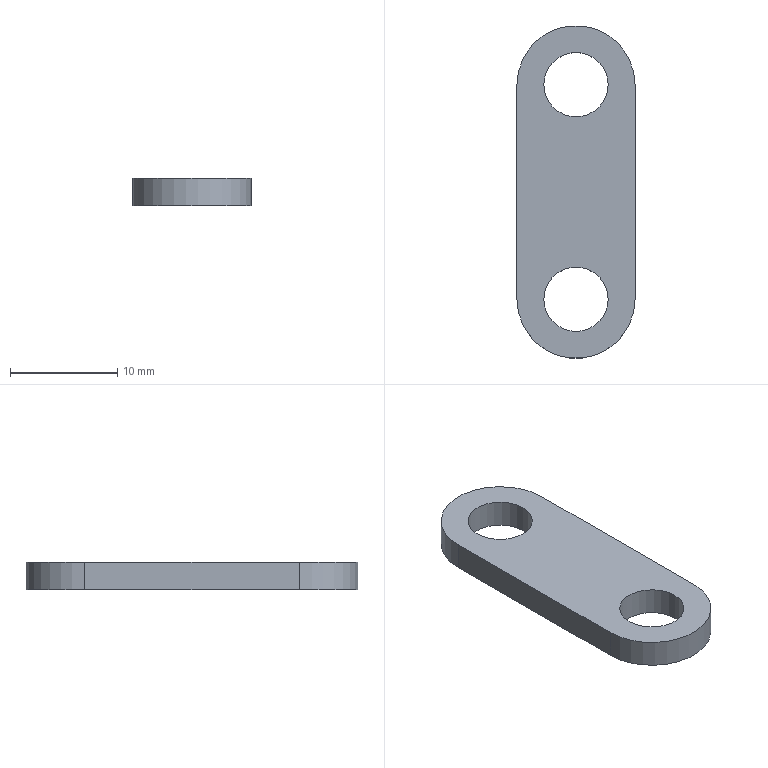Part | NX | features DATUM_CSYS 2, EXTRUDE 1, SKETCH 1 | 1 solid | 8 faces | box 11 x 31 x 2.6 mm | volume 672.06 mm3 | plane 4 | cylinder 4 | commonest cylinder face diameters 6 x2 11 x2
STEP:
#1=CARTESIAN_POINT('',(-5.5,10.,0.));
#2=VERTEX_POINT('',#1);
#3=CARTESIAN_POINT('',(-5.5,-10.,0.));
#4=VERTEX_POINT('',#3);
#5=CARTESIAN_POINT('',(-5.5,10.,0.));
#6=DIRECTION('',(0.,-1.,0.));
#7=VECTOR('',#6,1000.);
#8=LINE('',#5,#7);
#9=EDGE_CURVE('',#2,#4,#8,.T.);
#10=ORIENTED_EDGE('',*,*,#9,.T.);
#11=CARTESIAN_POINT('',(-5.5,-10.,2.6));
#12=VERTEX_POINT('',#11);
#13=CARTESIAN_POINT('',(-5.5,-10.,2.6));
#14=DIRECTION('',(0.,0.,-1.));
#15=VECTOR('',#14,1000.);
#16=LINE('',#13,#15);
#17=EDGE_CURVE('',#12,#4,#16,.T.);
#18=ORIENTED_EDGE('',*,*,#17,.F.);
#19=CARTESIAN_POINT('',(-5.5,10.,2.6));
#20=VERTEX_POINT('',#19);
#21=CARTESIAN_POINT('',(-5.5,10.,2.6));
#22=DIRECTION('',(0.,-1.,0.));
#23=VECTOR('',#22,1000.);
#24=LINE('',#21,#23);
#25=EDGE_CURVE('',#20,#12,#24,.T.);
#26=ORIENTED_EDGE('',*,*,#25,.F.);
#27=CARTESIAN_POINT('',(-5.5,10.,2.6));
#28=DIRECTION('',(0.,0.,-1.));
#29=VECTOR('',#28,1000.);
#30=LINE('',#27,#29);
#31=EDGE_CURVE('',#20,#2,#30,.T.);
#32=ORIENTED_EDGE('',*,*,#31,.T.);
#33=EDGE_LOOP('',(#10,#18,#26,#32));
#34=FACE_BOUND('',#33,.T.);
#35=CARTESIAN_POINT('',(-5.5,10.,2.6));
#36=DIRECTION('',(1.,0.,0.));
#37=DIRECTION('',(0.,0.,-1.));
#38=AXIS2_PLACEMENT_3D('',#35,#36,#37);
#39=PLANE('',#38);
#40=ADVANCED_FACE('',(#34),#39,.F.);
#41=CARTESIAN_POINT('',(5.5,-10.,0.));
#42=VERTEX_POINT('',#41);
#43=CARTESIAN_POINT('',(0.,-10.,0.));
#44=DIRECTION('',(0.,0.,1.));
#45=DIRECTION('',(1.,0.,0.));
#46=AXIS2_PLACEMENT_3D('',#43,#44,#45);
#47=CIRCLE('',#46,5.5);
#48=EDGE_CURVE('',#4,#42,#47,.T.);
#49=ORIENTED_EDGE('',*,*,#48,.T.);
#50=CARTESIAN_POINT('',(5.5,-10.,2.6));
#51=VERTEX_POINT('',#50);
#52=CARTESIAN_POINT('',(5.5,-10.,2.6));
#53=DIRECTION('',(0.,0.,-1.));
#54=VECTOR('',#53,1000.);
#55=LINE('',#52,#54);
#56=EDGE_CURVE('',#51,#42,#55,.T.);
#57=ORIENTED_EDGE('',*,*,#56,.F.);
#58=CARTESIAN_POINT('',(0.,-10.,2.6));
#59=DIRECTION('',(0.,0.,1.));
#60=DIRECTION('',(1.,0.,0.));
#61=AXIS2_PLACEMENT_3D('',#58,#59,#60);
#62=CIRCLE('',#61,5.5);
#63=EDGE_CURVE('',#12,#51,#62,.T.);
#64=ORIENTED_EDGE('',*,*,#63,.F.);
#65=ORIENTED_EDGE('',*,*,#17,.T.);
#66=EDGE_LOOP('',(#49,#57,#64,#65));
#67=FACE_BOUND('',#66,.T.);
#68=CARTESIAN_POINT('',(0.,-10.,2.6));
#69=DIRECTION('',(0.,0.,-1.));
#70=DIRECTION('',(-1.,0.,0.));
#71=AXIS2_PLACEMENT_3D('',#68,#69,#70);
#72=CYLINDRICAL_SURFACE('',#71,5.5);
#73=ADVANCED_FACE('',(#67),#72,.T.);
#74=CARTESIAN_POINT('',(5.5,10.,0.));
#75=VERTEX_POINT('',#74);
#76=CARTESIAN_POINT('',(5.5,-10.,0.));
#77=DIRECTION('',(0.,1.,0.));
#78=VECTOR('',#77,1000.);
#79=LINE('',#76,#78);
#80=EDGE_CURVE('',#42,#75,#79,.T.);
#81=ORIENTED_EDGE('',*,*,#80,.T.);
#82=CARTESIAN_POINT('',(5.5,10.,2.6));
#83=VERTEX_POINT('',#82);
#84=CARTESIAN_POINT('',(5.5,10.,2.6));
#85=DIRECTION('',(0.,0.,-1.));
#86=VECTOR('',#85,1000.);
#87=LINE('',#84,#86);
#88=EDGE_CURVE('',#83,#75,#87,.T.);
#89=ORIENTED_EDGE('',*,*,#88,.F.);
#90=CARTESIAN_POINT('',(5.5,-10.,2.6));
#91=DIRECTION('',(0.,1.,0.));
#92=VECTOR('',#91,1000.);
#93=LINE('',#90,#92);
#94=EDGE_CURVE('',#51,#83,#93,.T.);
#95=ORIENTED_EDGE('',*,*,#94,.F.);
#96=ORIENTED_EDGE('',*,*,#56,.T.);
#97=EDGE_LOOP('',(#81,#89,#95,#96));
#98=FACE_BOUND('',#97,.T.);
#99=CARTESIAN_POINT('',(5.5,-10.,2.6));
#100=DIRECTION('',(-1.,0.,0.));
#101=DIRECTION('',(0.,0.,1.));
#102=AXIS2_PLACEMENT_3D('',#99,#100,#101);
#103=PLANE('',#102);
#104=ADVANCED_FACE('',(#98),#103,.F.);
#105=CARTESIAN_POINT('',(3.,-10.,2.6));
#106=VERTEX_POINT('',#105);
#107=CARTESIAN_POINT('',(0.,-10.,2.6));
#108=DIRECTION('',(0.,0.,1.));
#109=DIRECTION('',(1.,0.,0.));
#110=AXIS2_PLACEMENT_3D('',#107,#108,#109);
#111=CIRCLE('',#110,3.);
#112=EDGE_CURVE('',#106,#106,#111,.T.);
#113=ORIENTED_EDGE('',*,*,#112,.T.);
#114=EDGE_LOOP('',(#113));
#115=FACE_BOUND('',#114,.T.);
#116=CARTESIAN_POINT('',(3.,-10.,0.));
#117=VERTEX_POINT('',#116);
#118=CARTESIAN_POINT('',(0.,-10.,0.));
#119=DIRECTION('',(0.,0.,1.));
#120=DIRECTION('',(1.,0.,0.));
#121=AXIS2_PLACEMENT_3D('',#118,#119,#120);
#122=CIRCLE('',#121,3.);
#123=EDGE_CURVE('',#117,#117,#122,.T.);
#124=ORIENTED_EDGE('',*,*,#123,.F.);
#125=EDGE_LOOP('',(#124));
#126=FACE_BOUND('',#125,.T.);
#127=CARTESIAN_POINT('',(0.,-10.,2.6));
#128=DIRECTION('',(0.,0.,-1.));
#129=DIRECTION('',(-1.,0.,0.));
#130=AXIS2_PLACEMENT_3D('',#127,#128,#129);
#131=CYLINDRICAL_SURFACE('',#130,3.);
#132=ADVANCED_FACE('',(#115,#126),#131,.F.);
#133=CARTESIAN_POINT('',(0.,10.,0.));
#134=DIRECTION('',(0.,0.,1.));
#135=DIRECTION('',(1.,0.,0.));
#136=AXIS2_PLACEMENT_3D('',#133,#134,#135);
#137=CIRCLE('',#136,5.5);
#138=EDGE_CURVE('',#75,#2,#137,.T.);
#139=ORIENTED_EDGE('',*,*,#138,.T.);
#140=ORIENTED_EDGE('',*,*,#31,.F.);
#141=CARTESIAN_POINT('',(0.,10.,2.6));
#142=DIRECTION('',(0.,0.,1.));
#143=DIRECTION('',(1.,0.,0.));
#144=AXIS2_PLACEMENT_3D('',#141,#142,#143);
#145=CIRCLE('',#144,5.5);
#146=EDGE_CURVE('',#83,#20,#145,.T.);
#147=ORIENTED_EDGE('',*,*,#146,.F.);
#148=ORIENTED_EDGE('',*,*,#88,.T.);
#149=EDGE_LOOP('',(#139,#140,#147,#148));
#150=FACE_BOUND('',#149,.T.);
#151=CARTESIAN_POINT('',(0.,10.,2.6));
#152=DIRECTION('',(0.,0.,-1.));
#153=DIRECTION('',(-1.,0.,0.));
#154=AXIS2_PLACEMENT_3D('',#151,#152,#153);
#155=CYLINDRICAL_SURFACE('',#154,5.5);
#156=ADVANCED_FACE('',(#150),#155,.T.);
#157=CARTESIAN_POINT('',(3.,10.,2.6));
#158=VERTEX_POINT('',#157);
#159=CARTESIAN_POINT('',(0.,10.,2.6));
#160=DIRECTION('',(0.,0.,1.));
#161=DIRECTION('',(1.,0.,0.));
#162=AXIS2_PLACEMENT_3D('',#159,#160,#161);
#163=CIRCLE('',#162,3.);
#164=EDGE_CURVE('',#158,#158,#163,.T.);
#165=ORIENTED_EDGE('',*,*,#164,.T.);
#166=EDGE_LOOP('',(#165));
#167=FACE_BOUND('',#166,.T.);
#168=CARTESIAN_POINT('',(3.,10.,0.));
#169=VERTEX_POINT('',#168);
#170=CARTESIAN_POINT('',(0.,10.,0.));
#171=DIRECTION('',(0.,0.,1.));
#172=DIRECTION('',(1.,0.,0.));
#173=AXIS2_PLACEMENT_3D('',#170,#171,#172);
#174=CIRCLE('',#173,3.);
#175=EDGE_CURVE('',#169,#169,#174,.T.);
#176=ORIENTED_EDGE('',*,*,#175,.F.);
#177=EDGE_LOOP('',(#176));
#178=FACE_BOUND('',#177,.T.);
#179=CARTESIAN_POINT('',(0.,10.,2.6));
#180=DIRECTION('',(0.,0.,-1.));
#181=DIRECTION('',(-1.,0.,0.));
#182=AXIS2_PLACEMENT_3D('',#179,#180,#181);
#183=CYLINDRICAL_SURFACE('',#182,3.);
#184=ADVANCED_FACE('',(#167,#178),#183,.F.);
#185=ORIENTED_EDGE('',*,*,#25,.T.);
#186=ORIENTED_EDGE('',*,*,#63,.T.);
#187=ORIENTED_EDGE('',*,*,#94,.T.);
#188=ORIENTED_EDGE('',*,*,#146,.T.);
#189=EDGE_LOOP('',(#185,#186,#187,#188));
#190=FACE_BOUND('',#189,.T.);
#191=ORIENTED_EDGE('',*,*,#112,.F.);
#192=EDGE_LOOP('',(#191));
#193=FACE_BOUND('',#192,.T.);
#194=ORIENTED_EDGE('',*,*,#164,.F.);
#195=EDGE_LOOP('',(#194));
#196=FACE_BOUND('',#195,.T.);
#197=CARTESIAN_POINT('',(0.,-10.,2.6));
#198=DIRECTION('',(0.,0.,1.));
#199=DIRECTION('',(1.,0.,0.));
#200=AXIS2_PLACEMENT_3D('',#197,#198,#199);
#201=PLANE('',#200);
#202=ADVANCED_FACE('',(#190,#193,#196),#201,.T.);
#203=ORIENTED_EDGE('',*,*,#9,.F.);
#204=ORIENTED_EDGE('',*,*,#138,.F.);
#205=ORIENTED_EDGE('',*,*,#80,.F.);
#206=ORIENTED_EDGE('',*,*,#48,.F.);
#207=EDGE_LOOP('',(#203,#204,#205,#206));
#208=FACE_BOUND('',#207,.T.);
#209=ORIENTED_EDGE('',*,*,#123,.T.);
#210=EDGE_LOOP('',(#209));
#211=FACE_BOUND('',#210,.T.);
#212=ORIENTED_EDGE('',*,*,#175,.T.);
#213=EDGE_LOOP('',(#212));
#214=FACE_BOUND('',#213,.T.);
#215=CARTESIAN_POINT('',(0.,-10.,0.));
#216=DIRECTION('',(0.,0.,1.));
#217=DIRECTION('',(1.,0.,0.));
#218=AXIS2_PLACEMENT_3D('',#215,#216,#217);
#219=PLANE('',#218);
#220=ADVANCED_FACE('',(#208,#211,#214),#219,.F.);
#221=CLOSED_SHELL('',(#40,#73,#104,#132,#156,#184,#202,#220));
#222=MANIFOLD_SOLID_BREP('',#221);
#223=(LENGTH_UNIT()NAMED_UNIT(*)SI_UNIT(.MILLI.,.METRE.));
#224=UNCERTAINTY_MEASURE_WITH_UNIT(LENGTH_MEASURE(0.00001),#223,'','');
#225=(NAMED_UNIT(*)PLANE_ANGLE_UNIT()SI_UNIT($,.RADIAN.));
#226=(NAMED_UNIT(*)SI_UNIT($,.STERADIAN.)SOLID_ANGLE_UNIT());
#227=(GEOMETRIC_REPRESENTATION_CONTEXT(3)GLOBAL_UNCERTAINTY_ASSIGNED_CONTEXT((#224))GLOBAL_UNIT_ASSIGNED_CONTEXT((#223,#225,#226))REPRESENTATION_CONTEXT('',''));
#228=ADVANCED_BREP_SHAPE_REPRESENTATION('',(#222),#227);